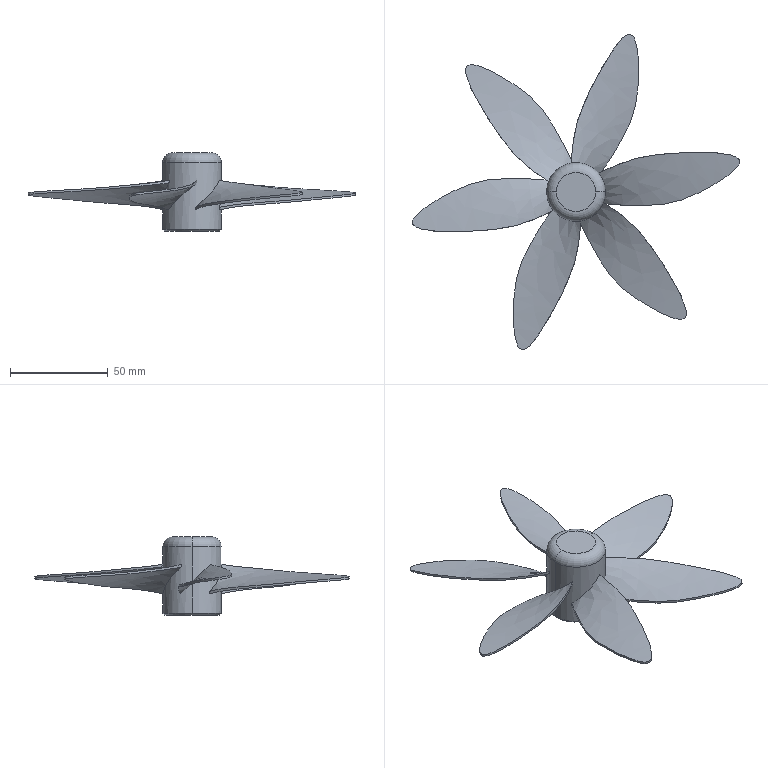Part | SolidWorks | 1 solid | 51 faces | box 167.128 x 160.8 x 40 mm | volume 32904 mm3 | spline 33 | plane 7 | cylinder 5 | cone 4 | torus 2 | commonest cylinder face diameters 20 x3 30 x2